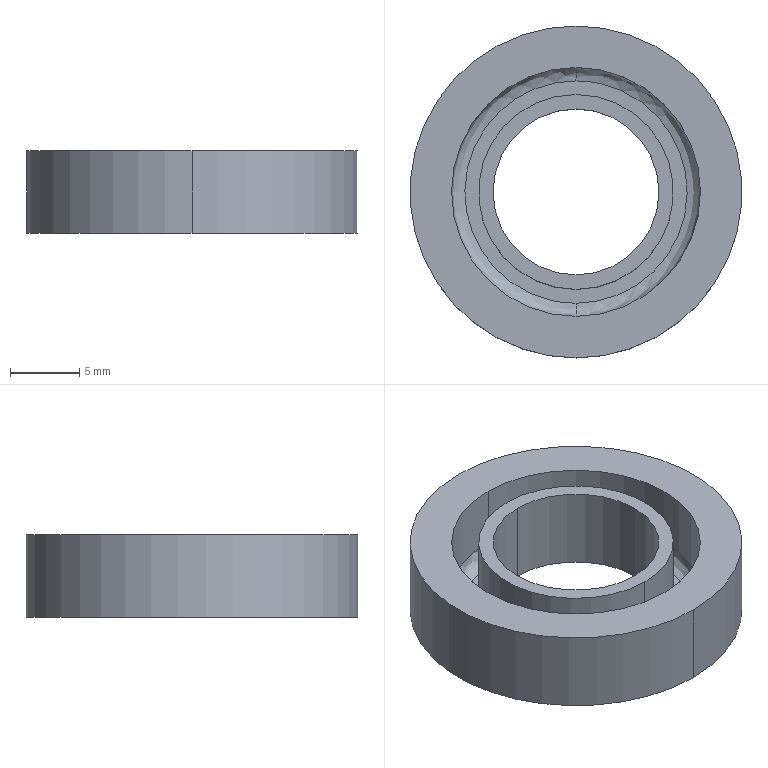Part | SolidWorks | features BaseBody 1 | 1 solid | 14 faces | box 24 x 24 x 6 mm | volume 1505 mm3 | cylinder 8 | plane 4 | spline 2 | commonest cylinder face diameters 12 x2 14.088 x2 18 x2 24 x2
STEP:
#1=CARTESIAN_POINT('',(0.,-8.038,1.5));
#2=VERTEX_POINT('',#1);
#3=CARTESIAN_POINT('',(0.,8.038,1.5));
#4=VERTEX_POINT('',#3);
#5=CARTESIAN_POINT('',(0.,-8.038,1.5));
#6=CARTESIAN_POINT('',(0.2456,-8.038,1.5));
#7=CARTESIAN_POINT('',(0.6127,-8.021,1.5));
#8=CARTESIAN_POINT('',(1.038,-7.972,1.5));
#9=CARTESIAN_POINT('',(1.251,-7.94,1.5));
#10=CARTESIAN_POINT('',(1.342,-7.925,1.5));
#11=CARTESIAN_POINT('',(1.402,-7.915,1.5));
#12=CARTESIAN_POINT('',(1.431,-7.909,1.5));
#13=CARTESIAN_POINT('',(1.719,-7.856,1.5));
#14=CARTESIAN_POINT('',(2.098,-7.767,1.5));
#15=CARTESIAN_POINT('',(2.531,-7.631,1.5));
#16=CARTESIAN_POINT('',(2.746,-7.555,1.5));
#17=CARTESIAN_POINT('',(2.837,-7.52,1.5));
#18=CARTESIAN_POINT('',(2.898,-7.497,1.5));
#19=CARTESIAN_POINT('',(2.927,-7.486,1.5));
#20=CARTESIAN_POINT('',(3.211,-7.373,1.5));
#21=CARTESIAN_POINT('',(3.58,-7.205,1.5));
#22=CARTESIAN_POINT('',(3.995,-6.977,1.5));
#23=CARTESIAN_POINT('',(4.169,-6.872,1.5));
#24=CARTESIAN_POINT('',(4.284,-6.801,1.5));
#25=CARTESIAN_POINT('',(4.34,-6.765,1.5));
#26=CARTESIAN_POINT('',(4.862,-6.424,1.5));
#27=CARTESIAN_POINT('',(5.291,-6.076,1.5));
#28=CARTESIAN_POINT('',(5.88,-5.487,1.5));
#29=CARTESIAN_POINT('',(6.157,-5.18,1.5));
#30=CARTESIAN_POINT('',(6.452,-4.797,1.5));
#31=CARTESIAN_POINT('',(6.572,-4.628,1.5));
#32=CARTESIAN_POINT('',(6.651,-4.514,1.5));
#33=CARTESIAN_POINT('',(6.69,-4.455,1.5));
#34=CARTESIAN_POINT('',(6.876,-4.171,1.5));
#35=CARTESIAN_POINT('',(7.081,-3.821,1.5));
#36=CARTESIAN_POINT('',(7.288,-3.395,1.5));
#37=CARTESIAN_POINT('',(7.383,-3.178,1.5));
#38=CARTESIAN_POINT('',(7.422,-3.084,1.5));
#39=CARTESIAN_POINT('',(7.448,-3.022,1.5));
#40=CARTESIAN_POINT('',(7.461,-2.989,1.5));
#41=CARTESIAN_POINT('',(7.569,-2.716,1.5));
#42=CARTESIAN_POINT('',(7.695,-2.348,1.5));
#43=CARTESIAN_POINT('',(7.81,-1.908,1.5));
#44=CARTESIAN_POINT('',(7.859,-1.686,1.5));
#45=CARTESIAN_POINT('',(7.879,-1.591,1.5));
#46=CARTESIAN_POINT('',(7.891,-1.527,1.5));
#47=CARTESIAN_POINT('',(7.898,-1.493,1.5));
#48=CARTESIAN_POINT('',(7.993,-0.9793,1.5));
#49=CARTESIAN_POINT('',(8.038,-0.4918,1.5));
#50=CARTESIAN_POINT('',(8.038,0.2459,1.5));
#51=CARTESIAN_POINT('',(8.027,0.4905,1.5));
#52=CARTESIAN_POINT('',(7.993,0.8561,1.5));
#53=CARTESIAN_POINT('',(7.972,1.039,1.5));
#54=CARTESIAN_POINT('',(7.94,1.251,1.5));
#55=CARTESIAN_POINT('',(7.925,1.342,1.5));
#56=CARTESIAN_POINT('',(7.915,1.402,1.5));
#57=CARTESIAN_POINT('',(7.909,1.431,1.5));
#58=CARTESIAN_POINT('',(7.856,1.719,1.5));
#59=CARTESIAN_POINT('',(7.767,2.098,1.5));
#60=CARTESIAN_POINT('',(7.631,2.531,1.5));
#61=CARTESIAN_POINT('',(7.555,2.746,1.5));
#62=CARTESIAN_POINT('',(7.52,2.837,1.5));
#63=CARTESIAN_POINT('',(7.497,2.898,1.5));
#64=CARTESIAN_POINT('',(7.486,2.927,1.5));
#65=CARTESIAN_POINT('',(7.373,3.211,1.5));
#66=CARTESIAN_POINT('',(7.205,3.58,1.5));
#67=CARTESIAN_POINT('',(6.977,3.995,1.5));
#68=CARTESIAN_POINT('',(6.872,4.169,1.5));
#69=CARTESIAN_POINT('',(6.801,4.284,1.5));
#70=CARTESIAN_POINT('',(6.765,4.34,1.5));
#71=CARTESIAN_POINT('',(6.424,4.862,1.5));
#72=CARTESIAN_POINT('',(6.076,5.291,1.5));
#73=CARTESIAN_POINT('',(5.487,5.88,1.5));
#74=CARTESIAN_POINT('',(5.18,6.157,1.5));
#75=CARTESIAN_POINT('',(4.797,6.452,1.5));
#76=CARTESIAN_POINT('',(4.628,6.572,1.5));
#77=CARTESIAN_POINT('',(4.514,6.651,1.5));
#78=CARTESIAN_POINT('',(4.455,6.69,1.5));
#79=CARTESIAN_POINT('',(4.171,6.876,1.5));
#80=CARTESIAN_POINT('',(3.821,7.081,1.5));
#81=CARTESIAN_POINT('',(3.395,7.288,1.5));
#82=CARTESIAN_POINT('',(3.178,7.383,1.5));
#83=CARTESIAN_POINT('',(3.084,7.422,1.5));
#84=CARTESIAN_POINT('',(3.022,7.448,1.5));
#85=CARTESIAN_POINT('',(2.989,7.461,1.5));
#86=CARTESIAN_POINT('',(2.716,7.569,1.5));
#87=CARTESIAN_POINT('',(2.348,7.695,1.5));
#88=CARTESIAN_POINT('',(1.908,7.81,1.5));
#89=CARTESIAN_POINT('',(1.686,7.859,1.5));
#90=CARTESIAN_POINT('',(1.591,7.879,1.5));
#91=CARTESIAN_POINT('',(1.527,7.891,1.5));
#92=CARTESIAN_POINT('',(1.493,7.898,1.5));
#93=CARTESIAN_POINT('',(0.9795,7.993,1.5));
#94=CARTESIAN_POINT('',(0.4913,8.038,1.5));
#95=CARTESIAN_POINT('',(0.,8.038,1.5));
#96=B_SPLINE_CURVE_WITH_KNOTS('',3,(#5,#6,#7,#8,#9,#10,#11,#12,#13,#14,#15,#16,#17,#18,#19,#20,#21,#22,#23,#24,#25,#26,#27,#28,#29,#30,#31,#32,#33,#34,#35,#36,#37,#38,#39,#40,#41,#42,#43,#44,#45,#46,#47,#48,#49,#50,#51,#52,#53,#54,#55,#56,#57,#58,#59,#60,#61,#62,#63,#64,#65,#66,#67,#68,#69,#70,#71,#72,#73,#74,#75,#76,#77,#78,#79,#80,#81,#82,#83,#84,#85,#86,#87,#88,#89,#90,#91,#92,#93,#94,#95),.UNSPECIFIED.,.F.,.F.,(4,1,1,1,2,2,1,1,1,2,2,1,1,2,2,2,1,1,2,2,1,1,1,2,2,1,1,1,2,2,2,2,1,1,2,2,1,1,1,2,2,1,1,2,2,2,1,1,2,2,1,1,1,2,2,1,1,1,2,2,4),(0.75,0.7656,0.7734,0.7773,0.7793,0.7812,0.7969,0.8047,0.8086,0.8105,0.8125,0.8281,0.8359,0.8398,0.8437,0.875,0.8906,0.8984,0.9023,0.9063,0.9219,0.9297,0.9336,0.9355,0.9375,0.9531,0.9609,0.9648,0.9668,0.9688,1.,1.016,1.023,1.027,1.029,1.031,1.047,1.055,1.059,1.061,1.062,1.078,1.086,1.09,1.094,1.125,1.141,1.148,1.152,1.156,1.172,1.18,1.184,1.186,1.187,1.203,1.211,1.215,1.217,1.219,1.25),.UNSPECIFIED.);
#97=EDGE_CURVE('',#2,#4,#96,.T.);
#98=ORIENTED_EDGE('',*,*,#97,.F.);
#99=CARTESIAN_POINT('',(0.,-9.,2.462));
#100=VERTEX_POINT('',#99);
#101=CARTESIAN_POINT('',(0.,-8.038,2.462));
#102=DIRECTION('',(-1.,0.,0.));
#103=DIRECTION('',(0.,-1.,0.));
#104=AXIS2_PLACEMENT_3D('',#101,#102,#103);
#105=CIRCLE('',#104,0.9623);
#106=EDGE_CURVE('',#2,#100,#105,.T.);
#107=ORIENTED_EDGE('',*,*,#106,.T.);
#108=CARTESIAN_POINT('',(0.,9.,2.462));
#109=VERTEX_POINT('',#108);
#110=CARTESIAN_POINT('',(0.,0.,2.462));
#111=DIRECTION('',(0.,0.,1.));
#112=DIRECTION('',(0.,1.,0.));
#113=AXIS2_PLACEMENT_3D('',#110,#111,#112);
#114=CIRCLE('',#113,9.);
#115=EDGE_CURVE('',#100,#109,#114,.T.);
#116=ORIENTED_EDGE('',*,*,#115,.T.);
#117=CARTESIAN_POINT('',(0.,8.038,2.462));
#118=DIRECTION('',(1.,0.,0.));
#119=DIRECTION('',(0.,1.,0.));
#120=AXIS2_PLACEMENT_3D('',#117,#118,#119);
#121=CIRCLE('',#120,0.9623);
#122=EDGE_CURVE('',#4,#109,#121,.T.);
#123=ORIENTED_EDGE('',*,*,#122,.F.);
#124=EDGE_LOOP('',(#98,#107,#116,#123));
#125=FACE_OUTER_BOUND('',#124,.T.);
#126=CARTESIAN_POINT('',(0.,8.038,1.5));
#127=CARTESIAN_POINT('',(16.075,8.038,1.5));
#128=CARTESIAN_POINT('',(16.075,-8.038,1.5));
#129=CARTESIAN_POINT('',(0.,-8.038,1.5));
#130=CARTESIAN_POINT('',(0.,8.601,1.5));
#131=CARTESIAN_POINT('',(17.203,8.601,1.5));
#132=CARTESIAN_POINT('',(17.203,-8.601,1.5));
#133=CARTESIAN_POINT('',(0.,-8.601,1.5));
#134=CARTESIAN_POINT('',(0.,9.,1.899));
#135=CARTESIAN_POINT('',(18.,9.,1.899));
#136=CARTESIAN_POINT('',(18.,-9.,1.899));
#137=CARTESIAN_POINT('',(0.,-9.,1.899));
#138=CARTESIAN_POINT('',(0.,9.,2.462));
#139=CARTESIAN_POINT('',(18.,9.,2.462));
#140=CARTESIAN_POINT('',(18.,-9.,2.462));
#141=CARTESIAN_POINT('',(0.,-9.,2.462));
#142=(BOUNDED_SURFACE()B_SPLINE_SURFACE(3,3,((#126,#127,#128,#129),(#130,#131,#132,#133),(#134,#135,#136,#137),(#138,#139,#140,#141)),.UNSPECIFIED.,.F.,.F.,.T.)B_SPLINE_SURFACE_WITH_KNOTS((4,4),(4,4),(0.,1.),(0.,1.),.UNSPECIFIED.)GEOMETRIC_REPRESENTATION_ITEM()RATIONAL_B_SPLINE_SURFACE(((1.,0.3333,0.3333,1.),(0.8047,0.2682,0.2682,0.8047),(0.8047,0.2682,0.2682,0.8047),(1.,0.3333,0.3333,1.)))REPRESENTATION_ITEM('')SURFACE());
#143=ADVANCED_FACE('',(#125),#142,.F.);
#144=CARTESIAN_POINT('',(0.,12.,7.));
#145=VERTEX_POINT('',#144);
#146=CARTESIAN_POINT('',(0.,-12.,7.));
#147=VERTEX_POINT('',#146);
#148=CARTESIAN_POINT('',(0.,0.,7.));
#149=DIRECTION('',(0.,0.,-1.));
#150=DIRECTION('',(0.,1.,0.));
#151=AXIS2_PLACEMENT_3D('',#148,#149,#150);
#152=CIRCLE('',#151,12.);
#153=EDGE_CURVE('',#145,#147,#152,.T.);
#154=ORIENTED_EDGE('',*,*,#153,.T.);
#155=CARTESIAN_POINT('',(0.,-12.,1.));
#156=VERTEX_POINT('',#155);
#157=CARTESIAN_POINT('',(0.,-12.,0.));
#158=DIRECTION('',(0.,0.,-1.));
#159=VECTOR('',#158,1000.);
#160=LINE('',#157,#159);
#161=EDGE_CURVE('',#147,#156,#160,.T.);
#162=ORIENTED_EDGE('',*,*,#161,.T.);
#163=CARTESIAN_POINT('',(0.,12.,1.));
#164=VERTEX_POINT('',#163);
#165=CARTESIAN_POINT('',(0.,0.,1.));
#166=DIRECTION('',(0.,0.,1.));
#167=DIRECTION('',(0.,1.,0.));
#168=AXIS2_PLACEMENT_3D('',#165,#166,#167);
#169=CIRCLE('',#168,12.);
#170=EDGE_CURVE('',#156,#164,#169,.T.);
#171=ORIENTED_EDGE('',*,*,#170,.T.);
#172=CARTESIAN_POINT('',(0.,12.,0.));
#173=DIRECTION('',(0.,0.,-1.));
#174=VECTOR('',#173,1000.);
#175=LINE('',#172,#174);
#176=EDGE_CURVE('',#145,#164,#175,.T.);
#177=ORIENTED_EDGE('',*,*,#176,.F.);
#178=EDGE_LOOP('',(#154,#162,#171,#177));
#179=FACE_OUTER_BOUND('',#178,.T.);
#180=CARTESIAN_POINT('',(0.,0.,0.));
#181=DIRECTION('',(0.,0.,-1.));
#182=DIRECTION('',(0.,1.,0.));
#183=AXIS2_PLACEMENT_3D('',#180,#181,#182);
#184=CYLINDRICAL_SURFACE('',#183,12.);
#185=ADVANCED_FACE('',(#179),#184,.T.);
#186=CARTESIAN_POINT('',(0.,-6.,7.));
#187=VERTEX_POINT('',#186);
#188=CARTESIAN_POINT('',(0.,6.,7.));
#189=VERTEX_POINT('',#188);
#190=CARTESIAN_POINT('',(0.,0.,7.));
#191=DIRECTION('',(0.,0.,-1.));
#192=DIRECTION('',(0.,1.,0.));
#193=AXIS2_PLACEMENT_3D('',#190,#191,#192);
#194=CIRCLE('',#193,6.);
#195=EDGE_CURVE('',#187,#189,#194,.T.);
#196=ORIENTED_EDGE('',*,*,#195,.F.);
#197=CARTESIAN_POINT('',(0.,-6.,1.));
#198=VERTEX_POINT('',#197);
#199=CARTESIAN_POINT('',(0.,-6.,0.));
#200=DIRECTION('',(0.,0.,-1.));
#201=VECTOR('',#200,1000.);
#202=LINE('',#199,#201);
#203=EDGE_CURVE('',#187,#198,#202,.T.);
#204=ORIENTED_EDGE('',*,*,#203,.T.);
#205=CARTESIAN_POINT('',(0.,6.,1.));
#206=VERTEX_POINT('',#205);
#207=CARTESIAN_POINT('',(0.,0.,1.));
#208=DIRECTION('',(0.,0.,1.));
#209=DIRECTION('',(0.,1.,0.));
#210=AXIS2_PLACEMENT_3D('',#207,#208,#209);
#211=CIRCLE('',#210,6.);
#212=EDGE_CURVE('',#206,#198,#211,.T.);
#213=ORIENTED_EDGE('',*,*,#212,.F.);
#214=CARTESIAN_POINT('',(0.,6.,0.));
#215=DIRECTION('',(0.,0.,-1.));
#216=VECTOR('',#215,1000.);
#217=LINE('',#214,#216);
#218=EDGE_CURVE('',#189,#206,#217,.T.);
#219=ORIENTED_EDGE('',*,*,#218,.F.);
#220=EDGE_LOOP('',(#196,#204,#213,#219));
#221=FACE_OUTER_BOUND('',#220,.T.);
#222=CARTESIAN_POINT('',(0.,0.,0.));
#223=DIRECTION('',(0.,0.,-1.));
#224=DIRECTION('',(0.,1.,0.));
#225=AXIS2_PLACEMENT_3D('',#222,#223,#224);
#226=CYLINDRICAL_SURFACE('',#225,6.);
#227=ADVANCED_FACE('',(#221),#226,.F.);
#228=CARTESIAN_POINT('',(0.,-9.,7.));
#229=VERTEX_POINT('',#228);
#230=CARTESIAN_POINT('',(0.,9.,7.));
#231=VERTEX_POINT('',#230);
#232=CARTESIAN_POINT('',(0.,0.,7.));
#233=DIRECTION('',(0.,0.,-1.));
#234=DIRECTION('',(0.,1.,0.));
#235=AXIS2_PLACEMENT_3D('',#232,#233,#234);
#236=CIRCLE('',#235,9.);
#237=EDGE_CURVE('',#229,#231,#236,.T.);
#238=ORIENTED_EDGE('',*,*,#237,.F.);
#239=CARTESIAN_POINT('',(0.,-9.,0.));
#240=DIRECTION('',(0.,0.,-1.));
#241=VECTOR('',#240,1000.);
#242=LINE('',#239,#241);
#243=EDGE_CURVE('',#229,#100,#242,.T.);
#244=ORIENTED_EDGE('',*,*,#243,.T.);
#245=CARTESIAN_POINT('',(0.,0.,2.462));
#246=DIRECTION('',(0.,0.,1.));
#247=DIRECTION('',(0.,1.,0.));
#248=AXIS2_PLACEMENT_3D('',#245,#246,#247);
#249=CIRCLE('',#248,9.);
#250=EDGE_CURVE('',#109,#100,#249,.T.);
#251=ORIENTED_EDGE('',*,*,#250,.F.);
#252=CARTESIAN_POINT('',(0.,9.,0.));
#253=DIRECTION('',(0.,0.,-1.));
#254=VECTOR('',#253,1000.);
#255=LINE('',#252,#254);
#256=EDGE_CURVE('',#231,#109,#255,.T.);
#257=ORIENTED_EDGE('',*,*,#256,.F.);
#258=EDGE_LOOP('',(#238,#244,#251,#257));
#259=FACE_OUTER_BOUND('',#258,.T.);
#260=CARTESIAN_POINT('',(0.,0.,0.));
#261=DIRECTION('',(0.,0.,-1.));
#262=DIRECTION('',(0.,1.,0.));
#263=AXIS2_PLACEMENT_3D('',#260,#261,#262);
#264=CYLINDRICAL_SURFACE('',#263,9.);
#265=ADVANCED_FACE('',(#259),#264,.F.);
#266=CARTESIAN_POINT('',(0.,-7.044,7.));
#267=VERTEX_POINT('',#266);
#268=CARTESIAN_POINT('',(0.,7.044,7.));
#269=VERTEX_POINT('',#268);
#270=CARTESIAN_POINT('',(0.,0.,7.));
#271=DIRECTION('',(0.,0.,1.));
#272=DIRECTION('',(0.,1.,0.));
#273=AXIS2_PLACEMENT_3D('',#270,#271,#272);
#274=CIRCLE('',#273,7.044);
#275=EDGE_CURVE('',#267,#269,#274,.T.);
#276=ORIENTED_EDGE('',*,*,#275,.F.);
#277=CARTESIAN_POINT('',(0.,-7.044,1.5));
#278=VERTEX_POINT('',#277);
#279=CARTESIAN_POINT('',(0.,-7.044,0.));
#280=DIRECTION('',(0.,0.,-1.));
#281=VECTOR('',#280,1000.);
#282=LINE('',#279,#281);
#283=EDGE_CURVE('',#267,#278,#282,.T.);
#284=ORIENTED_EDGE('',*,*,#283,.T.);
#285=CARTESIAN_POINT('',(0.,7.044,1.5));
#286=VERTEX_POINT('',#285);
#287=CARTESIAN_POINT('',(0.,0.,1.5));
#288=DIRECTION('',(0.,0.,1.));
#289=DIRECTION('',(0.,1.,0.));
#290=AXIS2_PLACEMENT_3D('',#287,#288,#289);
#291=CIRCLE('',#290,7.044);
#292=EDGE_CURVE('',#278,#286,#291,.T.);
#293=ORIENTED_EDGE('',*,*,#292,.T.);
#294=CARTESIAN_POINT('',(0.,7.044,0.));
#295=DIRECTION('',(0.,0.,-1.));
#296=VECTOR('',#295,1000.);
#297=LINE('',#294,#296);
#298=EDGE_CURVE('',#269,#286,#297,.T.);
#299=ORIENTED_EDGE('',*,*,#298,.F.);
#300=EDGE_LOOP('',(#276,#284,#293,#299));
#301=FACE_OUTER_BOUND('',#300,.T.);
#302=CARTESIAN_POINT('',(0.,0.,0.));
#303=DIRECTION('',(0.,0.,-1.));
#304=DIRECTION('',(0.,1.,0.));
#305=AXIS2_PLACEMENT_3D('',#302,#303,#304);
#306=CYLINDRICAL_SURFACE('',#305,7.044);
#307=ADVANCED_FACE('',(#301),#306,.T.);
#308=ORIENTED_EDGE('',*,*,#161,.F.);
#309=CARTESIAN_POINT('',(0.,0.,7.));
#310=DIRECTION('',(0.,0.,-1.));
#311=DIRECTION('',(0.,1.,0.));
#312=AXIS2_PLACEMENT_3D('',#309,#310,#311);
#313=CIRCLE('',#312,12.);
#314=EDGE_CURVE('',#147,#145,#313,.T.);
#315=ORIENTED_EDGE('',*,*,#314,.T.);
#316=ORIENTED_EDGE('',*,*,#176,.T.);
#317=CARTESIAN_POINT('',(0.,0.,1.));
#318=DIRECTION('',(0.,0.,1.));
#319=DIRECTION('',(0.,1.,0.));
#320=AXIS2_PLACEMENT_3D('',#317,#318,#319);
#321=CIRCLE('',#320,12.);
#322=EDGE_CURVE('',#164,#156,#321,.T.);
#323=ORIENTED_EDGE('',*,*,#322,.T.);
#324=EDGE_LOOP('',(#308,#315,#316,#323));
#325=FACE_OUTER_BOUND('',#324,.T.);
#326=CARTESIAN_POINT('',(0.,0.,0.));
#327=DIRECTION('',(0.,0.,-1.));
#328=DIRECTION('',(0.,1.,0.));
#329=AXIS2_PLACEMENT_3D('',#326,#327,#328);
#330=CYLINDRICAL_SURFACE('',#329,12.);
#331=ADVANCED_FACE('',(#325),#330,.T.);
#332=ORIENTED_EDGE('',*,*,#212,.T.);
#333=CARTESIAN_POINT('',(0.,0.,1.));
#334=DIRECTION('',(0.,0.,1.));
#335=DIRECTION('',(0.,1.,0.));
#336=AXIS2_PLACEMENT_3D('',#333,#334,#335);
#337=CIRCLE('',#336,6.);
#338=EDGE_CURVE('',#198,#206,#337,.T.);
#339=ORIENTED_EDGE('',*,*,#338,.T.);
#340=EDGE_LOOP('',(#332,#339));
#341=FACE_BOUND('',#340,.T.);
#342=ORIENTED_EDGE('',*,*,#322,.F.);
#343=ORIENTED_EDGE('',*,*,#170,.F.);
#344=EDGE_LOOP('',(#342,#343));
#345=FACE_OUTER_BOUND('',#344,.T.);
#346=CARTESIAN_POINT('',(6.,0.,1.));
#347=DIRECTION('',(0.,0.,-1.));
#348=DIRECTION('',(0.,1.,0.));
#349=AXIS2_PLACEMENT_3D('',#346,#347,#348);
#350=PLANE('',#349);
#351=ADVANCED_FACE('',(#341,#345),#350,.T.);
#352=ORIENTED_EDGE('',*,*,#153,.F.);
#353=ORIENTED_EDGE('',*,*,#314,.F.);
#354=EDGE_LOOP('',(#352,#353));
#355=FACE_OUTER_BOUND('',#354,.T.);
#356=CARTESIAN_POINT('',(0.,0.,7.));
#357=DIRECTION('',(0.,0.,-1.));
#358=DIRECTION('',(0.,1.,0.));
#359=AXIS2_PLACEMENT_3D('',#356,#357,#358);
#360=CIRCLE('',#359,9.);
#361=EDGE_CURVE('',#231,#229,#360,.T.);
#362=ORIENTED_EDGE('',*,*,#361,.T.);
#363=ORIENTED_EDGE('',*,*,#237,.T.);
#364=EDGE_LOOP('',(#362,#363));
#365=FACE_BOUND('',#364,.T.);
#366=CARTESIAN_POINT('',(12.,0.,7.));
#367=DIRECTION('',(0.,0.,1.));
#368=DIRECTION('',(0.,-1.,0.));
#369=AXIS2_PLACEMENT_3D('',#366,#367,#368);
#370=PLANE('',#369);
#371=ADVANCED_FACE('',(#355,#365),#370,.T.);
#372=ORIENTED_EDGE('',*,*,#203,.F.);
#373=CARTESIAN_POINT('',(0.,0.,7.));
#374=DIRECTION('',(0.,0.,-1.));
#375=DIRECTION('',(0.,1.,0.));
#376=AXIS2_PLACEMENT_3D('',#373,#374,#375);
#377=CIRCLE('',#376,6.);
#378=EDGE_CURVE('',#189,#187,#377,.T.);
#379=ORIENTED_EDGE('',*,*,#378,.F.);
#380=ORIENTED_EDGE('',*,*,#218,.T.);
#381=ORIENTED_EDGE('',*,*,#338,.F.);
#382=EDGE_LOOP('',(#372,#379,#380,#381));
#383=FACE_OUTER_BOUND('',#382,.T.);
#384=CARTESIAN_POINT('',(0.,0.,0.));
#385=DIRECTION('',(0.,0.,-1.));
#386=DIRECTION('',(0.,1.,0.));
#387=AXIS2_PLACEMENT_3D('',#384,#385,#386);
#388=CYLINDRICAL_SURFACE('',#387,6.);
#389=ADVANCED_FACE('',(#383),#388,.F.);
#390=ORIENTED_EDGE('',*,*,#243,.F.);
#391=ORIENTED_EDGE('',*,*,#361,.F.);
#392=ORIENTED_EDGE('',*,*,#256,.T.);
#393=ORIENTED_EDGE('',*,*,#115,.F.);
#394=EDGE_LOOP('',(#390,#391,#392,#393));
#395=FACE_OUTER_BOUND('',#394,.T.);
#396=CARTESIAN_POINT('',(0.,0.,0.));
#397=DIRECTION('',(0.,0.,-1.));
#398=DIRECTION('',(0.,1.,0.));
#399=AXIS2_PLACEMENT_3D('',#396,#397,#398);
#400=CYLINDRICAL_SURFACE('',#399,9.);
#401=ADVANCED_FACE('',(#395),#400,.F.);
#402=CARTESIAN_POINT('',(0.,0.,7.));
#403=DIRECTION('',(0.,0.,1.));
#404=DIRECTION('',(0.,1.,0.));
#405=AXIS2_PLACEMENT_3D('',#402,#403,#404);
#406=CIRCLE('',#405,7.044);
#407=EDGE_CURVE('',#269,#267,#406,.T.);
#408=ORIENTED_EDGE('',*,*,#407,.T.);
#409=ORIENTED_EDGE('',*,*,#275,.T.);
#410=EDGE_LOOP('',(#408,#409));
#411=FACE_OUTER_BOUND('',#410,.T.);
#412=ORIENTED_EDGE('',*,*,#378,.T.);
#413=ORIENTED_EDGE('',*,*,#195,.T.);
#414=EDGE_LOOP('',(#412,#413));
#415=FACE_BOUND('',#414,.T.);
#416=CARTESIAN_POINT('',(7.044,0.,7.));
#417=DIRECTION('',(0.,0.,1.));
#418=DIRECTION('',(0.,-1.,0.));
#419=AXIS2_PLACEMENT_3D('',#416,#417,#418);
#420=PLANE('',#419);
#421=ADVANCED_FACE('',(#411,#415),#420,.T.);
#422=ORIENTED_EDGE('',*,*,#106,.F.);
#423=CARTESIAN_POINT('',(0.,8.038,1.5));
#424=CARTESIAN_POINT('',(-0.2456,8.038,1.5));
#425=CARTESIAN_POINT('',(-0.6127,8.021,1.5));
#426=CARTESIAN_POINT('',(-1.038,7.972,1.5));
#427=CARTESIAN_POINT('',(-1.251,7.94,1.5));
#428=CARTESIAN_POINT('',(-1.342,7.925,1.5));
#429=CARTESIAN_POINT('',(-1.402,7.915,1.5));
#430=CARTESIAN_POINT('',(-1.431,7.909,1.5));
#431=CARTESIAN_POINT('',(-1.719,7.856,1.5));
#432=CARTESIAN_POINT('',(-2.098,7.767,1.5));
#433=CARTESIAN_POINT('',(-2.531,7.631,1.5));
#434=CARTESIAN_POINT('',(-2.746,7.555,1.5));
#435=CARTESIAN_POINT('',(-2.837,7.52,1.5));
#436=CARTESIAN_POINT('',(-2.898,7.497,1.5));
#437=CARTESIAN_POINT('',(-2.927,7.486,1.5));
#438=CARTESIAN_POINT('',(-3.211,7.373,1.5));
#439=CARTESIAN_POINT('',(-3.58,7.205,1.5));
#440=CARTESIAN_POINT('',(-3.995,6.977,1.5));
#441=CARTESIAN_POINT('',(-4.169,6.872,1.5));
#442=CARTESIAN_POINT('',(-4.284,6.801,1.5));
#443=CARTESIAN_POINT('',(-4.34,6.765,1.5));
#444=CARTESIAN_POINT('',(-4.862,6.424,1.5));
#445=CARTESIAN_POINT('',(-5.291,6.076,1.5));
#446=CARTESIAN_POINT('',(-5.88,5.487,1.5));
#447=CARTESIAN_POINT('',(-6.157,5.18,1.5));
#448=CARTESIAN_POINT('',(-6.452,4.797,1.5));
#449=CARTESIAN_POINT('',(-6.572,4.628,1.5));
#450=CARTESIAN_POINT('',(-6.651,4.514,1.5));
#451=CARTESIAN_POINT('',(-6.69,4.455,1.5));
#452=CARTESIAN_POINT('',(-6.876,4.171,1.5));
#453=CARTESIAN_POINT('',(-7.081,3.821,1.5));
#454=CARTESIAN_POINT('',(-7.288,3.395,1.5));
#455=CARTESIAN_POINT('',(-7.383,3.178,1.5));
#456=CARTESIAN_POINT('',(-7.422,3.084,1.5));
#457=CARTESIAN_POINT('',(-7.448,3.022,1.5));
#458=CARTESIAN_POINT('',(-7.461,2.989,1.5));
#459=CARTESIAN_POINT('',(-7.569,2.716,1.5));
#460=CARTESIAN_POINT('',(-7.695,2.348,1.5));
#461=CARTESIAN_POINT('',(-7.81,1.908,1.5));
#462=CARTESIAN_POINT('',(-7.859,1.686,1.5));
#463=CARTESIAN_POINT('',(-7.879,1.591,1.5));
#464=CARTESIAN_POINT('',(-7.891,1.527,1.5));
#465=CARTESIAN_POINT('',(-7.898,1.493,1.5));
#466=CARTESIAN_POINT('',(-7.993,0.9795,1.5));
#467=CARTESIAN_POINT('',(-8.038,0.4913,1.5));
#468=CARTESIAN_POINT('',(-8.038,-0.2456,1.5));
#469=CARTESIAN_POINT('',(-8.021,-0.6127,1.5));
#470=CARTESIAN_POINT('',(-7.972,-1.038,1.5));
#471=CARTESIAN_POINT('',(-7.94,-1.251,1.5));
#472=CARTESIAN_POINT('',(-7.925,-1.342,1.5));
#473=CARTESIAN_POINT('',(-7.915,-1.402,1.5));
#474=CARTESIAN_POINT('',(-7.909,-1.431,1.5));
#475=CARTESIAN_POINT('',(-7.856,-1.719,1.5));
#476=CARTESIAN_POINT('',(-7.767,-2.098,1.5));
#477=CARTESIAN_POINT('',(-7.631,-2.531,1.5));
#478=CARTESIAN_POINT('',(-7.555,-2.746,1.5));
#479=CARTESIAN_POINT('',(-7.52,-2.837,1.5));
#480=CARTESIAN_POINT('',(-7.497,-2.898,1.5));
#481=CARTESIAN_POINT('',(-7.486,-2.927,1.5));
#482=CARTESIAN_POINT('',(-7.373,-3.211,1.5));
#483=CARTESIAN_POINT('',(-7.205,-3.58,1.5));
#484=CARTESIAN_POINT('',(-6.977,-3.995,1.5));
#485=CARTESIAN_POINT('',(-6.872,-4.169,1.5));
#486=CARTESIAN_POINT('',(-6.801,-4.284,1.5));
#487=CARTESIAN_POINT('',(-6.765,-4.34,1.5));
#488=CARTESIAN_POINT('',(-6.424,-4.862,1.5));
#489=CARTESIAN_POINT('',(-6.076,-5.291,1.5));
#490=CARTESIAN_POINT('',(-5.487,-5.88,1.5));
#491=CARTESIAN_POINT('',(-5.18,-6.157,1.5));
#492=CARTESIAN_POINT('',(-4.797,-6.452,1.5));
#493=CARTESIAN_POINT('',(-4.628,-6.572,1.5));
#494=CARTESIAN_POINT('',(-4.514,-6.651,1.5));
#495=CARTESIAN_POINT('',(-4.455,-6.69,1.5));
#496=CARTESIAN_POINT('',(-4.171,-6.876,1.5));
#497=CARTESIAN_POINT('',(-3.821,-7.081,1.5));
#498=CARTESIAN_POINT('',(-3.395,-7.288,1.5));
#499=CARTESIAN_POINT('',(-3.178,-7.383,1.5));
#500=CARTESIAN_POINT('',(-3.084,-7.422,1.5));
#501=CARTESIAN_POINT('',(-3.022,-7.448,1.5));
#502=CARTESIAN_POINT('',(-2.989,-7.461,1.5));
#503=CARTESIAN_POINT('',(-2.716,-7.569,1.5));
#504=CARTESIAN_POINT('',(-2.348,-7.695,1.5));
#505=CARTESIAN_POINT('',(-1.908,-7.81,1.5));
#506=CARTESIAN_POINT('',(-1.686,-7.859,1.5));
#507=CARTESIAN_POINT('',(-1.591,-7.879,1.5));
#508=CARTESIAN_POINT('',(-1.527,-7.891,1.5));
#509=CARTESIAN_POINT('',(-1.493,-7.898,1.5));
#510=CARTESIAN_POINT('',(-0.9795,-7.993,1.5));
#511=CARTESIAN_POINT('',(-0.4913,-8.038,1.5));
#512=CARTESIAN_POINT('',(0.,-8.038,1.5));
#513=B_SPLINE_CURVE_WITH_KNOTS('',3,(#423,#424,#425,#426,#427,#428,#429,#430,#431,#432,#433,#434,#435,#436,#437,#438,#439,#440,#441,#442,#443,#444,#445,#446,#447,#448,#449,#450,#451,#452,#453,#454,#455,#456,#457,#458,#459,#460,#461,#462,#463,#464,#465,#466,#467,#468,#469,#470,#471,#472,#473,#474,#475,#476,#477,#478,#479,#480,#481,#482,#483,#484,#485,#486,#487,#488,#489,#490,#491,#492,#493,#494,#495,#496,#497,#498,#499,#500,#501,#502,#503,#504,#505,#506,#507,#508,#509,#510,#511,#512),.UNSPECIFIED.,.F.,.F.,(4,1,1,1,2,2,1,1,1,2,2,1,1,2,2,2,1,1,2,2,1,1,1,2,2,1,1,1,2,2,2,1,1,1,2,2,1,1,1,2,2,1,1,2,2,2,1,1,2,2,1,1,1,2,2,1,1,1,2,2,4),(0.25,0.2656,0.2734,0.2773,0.2793,0.2812,0.2969,0.3047,0.3086,0.3105,0.3125,0.3281,0.3359,0.3398,0.3438,0.375,0.3906,0.3984,0.4023,0.4063,0.4219,0.4297,0.4336,0.4355,0.4375,0.4531,0.4609,0.4648,0.4668,0.4687,0.5,0.5156,0.5234,0.5273,0.5293,0.5312,0.5469,0.5547,0.5586,0.5605,0.5625,0.5781,0.5859,0.5898,0.5938,0.625,0.6406,0.6484,0.6523,0.6562,0.6719,0.6797,0.6836,0.6855,0.6875,0.7031,0.7109,0.7148,0.7168,0.7188,0.75),.UNSPECIFIED.);
#514=EDGE_CURVE('',#4,#2,#513,.T.);
#515=ORIENTED_EDGE('',*,*,#514,.F.);
#516=ORIENTED_EDGE('',*,*,#122,.T.);
#517=ORIENTED_EDGE('',*,*,#250,.T.);
#518=EDGE_LOOP('',(#422,#515,#516,#517));
#519=FACE_OUTER_BOUND('',#518,.T.);
#520=CARTESIAN_POINT('',(0.,-8.038,1.5));
#521=CARTESIAN_POINT('',(-16.075,-8.038,1.5));
#522=CARTESIAN_POINT('',(-16.075,8.038,1.5));
#523=CARTESIAN_POINT('',(0.,8.038,1.5));
#524=CARTESIAN_POINT('',(0.,-8.601,1.5));
#525=CARTESIAN_POINT('',(-17.203,-8.601,1.5));
#526=CARTESIAN_POINT('',(-17.203,8.601,1.5));
#527=CARTESIAN_POINT('',(0.,8.601,1.5));
#528=CARTESIAN_POINT('',(0.,-9.,1.899));
#529=CARTESIAN_POINT('',(-18.,-9.,1.899));
#530=CARTESIAN_POINT('',(-18.,9.,1.899));
#531=CARTESIAN_POINT('',(0.,9.,1.899));
#532=CARTESIAN_POINT('',(0.,-9.,2.462));
#533=CARTESIAN_POINT('',(-18.,-9.,2.462));
#534=CARTESIAN_POINT('',(-18.,9.,2.462));
#535=CARTESIAN_POINT('',(0.,9.,2.462));
#536=(BOUNDED_SURFACE()B_SPLINE_SURFACE(3,3,((#520,#521,#522,#523),(#524,#525,#526,#527),(#528,#529,#530,#531),(#532,#533,#534,#535)),.UNSPECIFIED.,.F.,.F.,.F.)B_SPLINE_SURFACE_WITH_KNOTS((4,4),(4,4),(0.,1.),(0.,1.),.UNSPECIFIED.)GEOMETRIC_REPRESENTATION_ITEM()RATIONAL_B_SPLINE_SURFACE(((1.,0.3333,0.3333,1.),(0.8047,0.2682,0.2682,0.8047),(0.8047,0.2682,0.2682,0.8047),(1.,0.3333,0.3333,1.)))REPRESENTATION_ITEM('')SURFACE());
#537=ADVANCED_FACE('',(#519),#536,.F.);
#538=ORIENTED_EDGE('',*,*,#283,.F.);
#539=ORIENTED_EDGE('',*,*,#407,.F.);
#540=ORIENTED_EDGE('',*,*,#298,.T.);
#541=CARTESIAN_POINT('',(0.,0.,1.5));
#542=DIRECTION('',(0.,0.,1.));
#543=DIRECTION('',(0.,1.,0.));
#544=AXIS2_PLACEMENT_3D('',#541,#542,#543);
#545=CIRCLE('',#544,7.044);
#546=EDGE_CURVE('',#286,#278,#545,.T.);
#547=ORIENTED_EDGE('',*,*,#546,.T.);
#548=EDGE_LOOP('',(#538,#539,#540,#547));
#549=FACE_OUTER_BOUND('',#548,.T.);
#550=CARTESIAN_POINT('',(0.,0.,0.));
#551=DIRECTION('',(0.,0.,-1.));
#552=DIRECTION('',(0.,1.,0.));
#553=AXIS2_PLACEMENT_3D('',#550,#551,#552);
#554=CYLINDRICAL_SURFACE('',#553,7.044);
#555=ADVANCED_FACE('',(#549),#554,.T.);
#556=ORIENTED_EDGE('',*,*,#514,.T.);
#557=ORIENTED_EDGE('',*,*,#97,.T.);
#558=EDGE_LOOP('',(#556,#557));
#559=FACE_OUTER_BOUND('',#558,.T.);
#560=ORIENTED_EDGE('',*,*,#546,.F.);
#561=ORIENTED_EDGE('',*,*,#292,.F.);
#562=EDGE_LOOP('',(#560,#561));
#563=FACE_BOUND('',#562,.T.);
#564=CARTESIAN_POINT('',(8.038,0.,1.5));
#565=DIRECTION('',(0.,0.,1.));
#566=DIRECTION('',(0.,-1.,0.));
#567=AXIS2_PLACEMENT_3D('',#564,#565,#566);
#568=PLANE('',#567);
#569=ADVANCED_FACE('',(#559,#563),#568,.T.);
#570=CLOSED_SHELL('',(#143,#185,#227,#265,#307,#331,#351,#371,#389,#401,#421,#537,#555,#569));
#571=MANIFOLD_SOLID_BREP('',#570);
#572=CARTESIAN_POINT('',(0.,0.,0.));
#573=DIRECTION('',(0.,0.,1.));
#574=DIRECTION('',(1.,0.,0.));
#575=AXIS2_PLACEMENT_3D('',#572,#573,#574);
#576=(LENGTH_UNIT()NAMED_UNIT(*)SI_UNIT(.MILLI.,.METRE.));
#577=UNCERTAINTY_MEASURE_WITH_UNIT(LENGTH_MEASURE(0.00001),#576,'','');
#578=(NAMED_UNIT(*)PLANE_ANGLE_UNIT()SI_UNIT($,.RADIAN.));
#579=(NAMED_UNIT(*)SI_UNIT($,.STERADIAN.)SOLID_ANGLE_UNIT());
#580=(GEOMETRIC_REPRESENTATION_CONTEXT(3)GLOBAL_UNCERTAINTY_ASSIGNED_CONTEXT((#577))GLOBAL_UNIT_ASSIGNED_CONTEXT((#576,#578,#579))REPRESENTATION_CONTEXT('',''));
#581=ADVANCED_BREP_SHAPE_REPRESENTATION('',(#571,#575),#580);